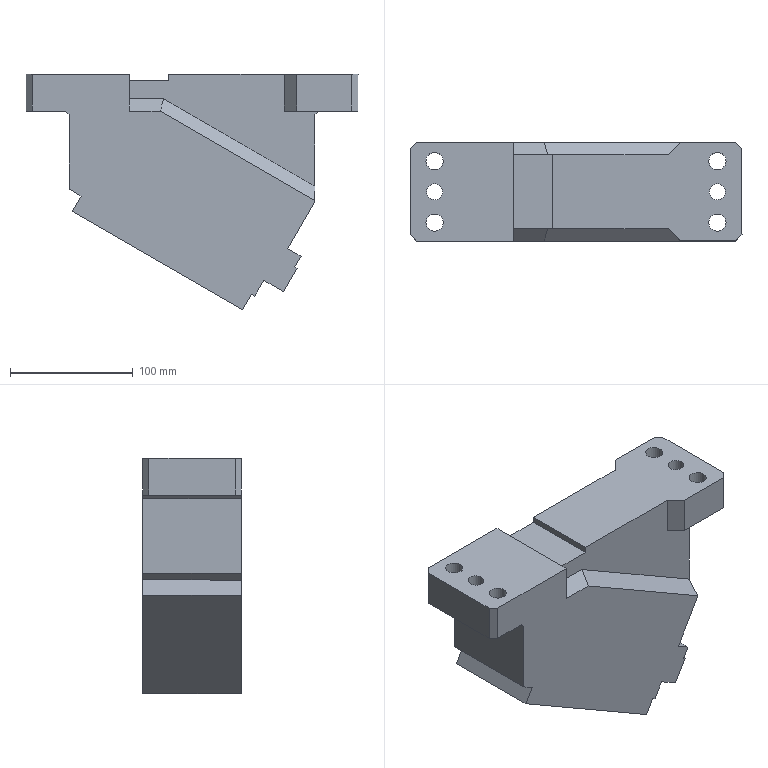Part | NX | features solid 2 | 1 solid | 55 faces | box 270.003 x 80.033 x 191.547 mm | volume 2416391 mm3 | plane 45 | cylinder 10 | commonest cylinder face diameters 14 x4 20 x4 13 x2